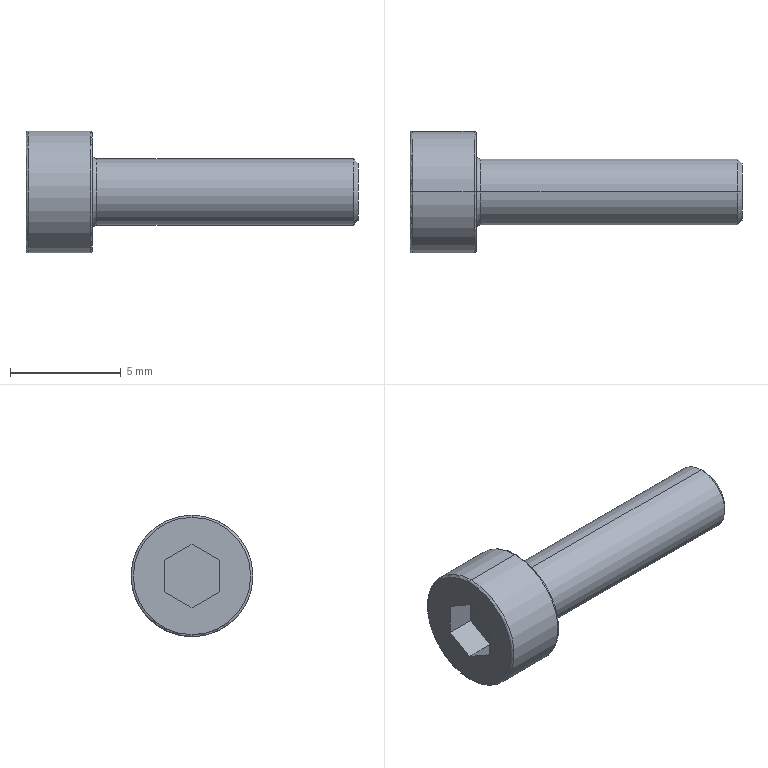Part | SolidWorks | features BlendCut 1, Chamfer 1, Cut 1, Fillet 1, Revolution 1 | 1 solid | 22 faces | box 15 x 5.5 x 5.5 mm | volume 148.972 mm3 | plane 10 | torus 6 | cylinder 4 | cone 2 | commonest cylinder face diameters 3 x2 5.5 x2
STEP:
#1=CARTESIAN_POINT('',(15.,0.,-1.3));
#2=VERTEX_POINT('',#1);
#3=CARTESIAN_POINT('',(15.,0.,1.3));
#4=VERTEX_POINT('',#3);
#5=CARTESIAN_POINT('',(15.,0.,0.));
#6=DIRECTION('',(1.,0.,0.));
#7=DIRECTION('',(0.,0.,1.));
#8=AXIS2_PLACEMENT_3D('',#5,#6,#7);
#9=CIRCLE('',#8,1.3);
#10=EDGE_CURVE('',#2,#4,#9,.T.);
#11=ORIENTED_EDGE('',*,*,#10,.F.);
#12=CARTESIAN_POINT('',(14.8,0.,-1.5));
#13=VERTEX_POINT('',#12);
#14=CARTESIAN_POINT('',(14.8,0.,-1.5));
#15=DIRECTION('',(-0.7071,0.,-0.7071));
#16=VECTOR('',#15,1000.);
#17=LINE('',#14,#16);
#18=EDGE_CURVE('',#2,#13,#17,.T.);
#19=ORIENTED_EDGE('',*,*,#18,.T.);
#20=CARTESIAN_POINT('',(14.8,0.,1.5));
#21=VERTEX_POINT('',#20);
#22=CARTESIAN_POINT('',(14.8,0.,0.));
#23=DIRECTION('',(-1.,0.,0.));
#24=DIRECTION('',(0.,0.,1.));
#25=AXIS2_PLACEMENT_3D('',#22,#23,#24);
#26=CIRCLE('',#25,1.5);
#27=EDGE_CURVE('',#21,#13,#26,.T.);
#28=ORIENTED_EDGE('',*,*,#27,.F.);
#29=CARTESIAN_POINT('',(14.8,0.,1.5));
#30=DIRECTION('',(-0.7071,0.,0.7071));
#31=VECTOR('',#30,1000.);
#32=LINE('',#29,#31);
#33=EDGE_CURVE('',#4,#21,#32,.T.);
#34=ORIENTED_EDGE('',*,*,#33,.F.);
#35=EDGE_LOOP('',(#11,#19,#28,#34));
#36=FACE_OUTER_BOUND('',#35,.T.);
#37=CARTESIAN_POINT('',(14.8,0.,0.));
#38=DIRECTION('',(-1.,0.,0.));
#39=DIRECTION('',(0.,0.,1.));
#40=AXIS2_PLACEMENT_3D('',#37,#38,#39);
#41=CONICAL_SURFACE('',#40,1.5,0.7854);
#42=ADVANCED_FACE('',(#36),#41,.T.);
#43=CARTESIAN_POINT('',(0.,0.,2.65));
#44=VERTEX_POINT('',#43);
#45=CARTESIAN_POINT('',(0.,0.,-2.65));
#46=VERTEX_POINT('',#45);
#47=CARTESIAN_POINT('',(0.,0.,0.));
#48=DIRECTION('',(-1.,0.,0.));
#49=DIRECTION('',(0.,0.,-1.));
#50=AXIS2_PLACEMENT_3D('',#47,#48,#49);
#51=CIRCLE('',#50,2.65);
#52=EDGE_CURVE('',#44,#46,#51,.T.);
#53=ORIENTED_EDGE('',*,*,#52,.F.);
#54=CARTESIAN_POINT('',(0.1,0.,2.75));
#55=VERTEX_POINT('',#54);
#56=CARTESIAN_POINT('',(0.1,0.,2.65));
#57=DIRECTION('',(0.,1.,0.));
#58=DIRECTION('',(0.,0.,1.));
#59=AXIS2_PLACEMENT_3D('',#56,#57,#58);
#60=CIRCLE('',#59,0.1);
#61=EDGE_CURVE('',#44,#55,#60,.T.);
#62=ORIENTED_EDGE('',*,*,#61,.T.);
#63=CARTESIAN_POINT('',(0.1,0.,-2.75));
#64=VERTEX_POINT('',#63);
#65=CARTESIAN_POINT('',(0.1,0.,0.));
#66=DIRECTION('',(1.,0.,0.));
#67=DIRECTION('',(0.,0.,-1.));
#68=AXIS2_PLACEMENT_3D('',#65,#66,#67);
#69=CIRCLE('',#68,2.75);
#70=EDGE_CURVE('',#64,#55,#69,.T.);
#71=ORIENTED_EDGE('',*,*,#70,.F.);
#72=CARTESIAN_POINT('',(0.1,0.,-2.65));
#73=DIRECTION('',(0.,-1.,0.));
#74=DIRECTION('',(0.,0.,-1.));
#75=AXIS2_PLACEMENT_3D('',#72,#73,#74);
#76=CIRCLE('',#75,0.1);
#77=EDGE_CURVE('',#46,#64,#76,.T.);
#78=ORIENTED_EDGE('',*,*,#77,.F.);
#79=EDGE_LOOP('',(#53,#62,#71,#78));
#80=FACE_OUTER_BOUND('',#79,.T.);
#81=CARTESIAN_POINT('',(0.1,0.,0.));
#82=DIRECTION('',(1.,0.,0.));
#83=DIRECTION('',(0.,0.,-1.));
#84=AXIS2_PLACEMENT_3D('',#81,#82,#83);
#85=TOROIDAL_SURFACE('',#84,2.65,0.1);
#86=ADVANCED_FACE('',(#80),#85,.T.);
#87=CARTESIAN_POINT('',(3.,0.,-2.65));
#88=VERTEX_POINT('',#87);
#89=CARTESIAN_POINT('',(3.,0.,2.65));
#90=VERTEX_POINT('',#89);
#91=CARTESIAN_POINT('',(3.,0.,0.));
#92=DIRECTION('',(1.,0.,0.));
#93=DIRECTION('',(0.,0.,1.));
#94=AXIS2_PLACEMENT_3D('',#91,#92,#93);
#95=CIRCLE('',#94,2.65);
#96=EDGE_CURVE('',#88,#90,#95,.T.);
#97=ORIENTED_EDGE('',*,*,#96,.F.);
#98=CARTESIAN_POINT('',(2.9,0.,-2.75));
#99=VERTEX_POINT('',#98);
#100=CARTESIAN_POINT('',(2.9,0.,-2.65));
#101=DIRECTION('',(0.,1.,0.));
#102=DIRECTION('',(0.,0.,1.));
#103=AXIS2_PLACEMENT_3D('',#100,#101,#102);
#104=CIRCLE('',#103,0.1);
#105=EDGE_CURVE('',#88,#99,#104,.T.);
#106=ORIENTED_EDGE('',*,*,#105,.T.);
#107=CARTESIAN_POINT('',(2.9,0.,2.75));
#108=VERTEX_POINT('',#107);
#109=CARTESIAN_POINT('',(2.9,0.,0.));
#110=DIRECTION('',(-1.,0.,0.));
#111=DIRECTION('',(0.,0.,1.));
#112=AXIS2_PLACEMENT_3D('',#109,#110,#111);
#113=CIRCLE('',#112,2.75);
#114=EDGE_CURVE('',#108,#99,#113,.T.);
#115=ORIENTED_EDGE('',*,*,#114,.F.);
#116=CARTESIAN_POINT('',(2.9,0.,2.65));
#117=DIRECTION('',(0.,-1.,0.));
#118=DIRECTION('',(0.,0.,-1.));
#119=AXIS2_PLACEMENT_3D('',#116,#117,#118);
#120=CIRCLE('',#119,0.1);
#121=EDGE_CURVE('',#90,#108,#120,.T.);
#122=ORIENTED_EDGE('',*,*,#121,.F.);
#123=EDGE_LOOP('',(#97,#106,#115,#122));
#124=FACE_OUTER_BOUND('',#123,.T.);
#125=CARTESIAN_POINT('',(2.9,0.,0.));
#126=DIRECTION('',(-1.,0.,0.));
#127=DIRECTION('',(0.,0.,1.));
#128=AXIS2_PLACEMENT_3D('',#125,#126,#127);
#129=TOROIDAL_SURFACE('',#128,2.65,0.1);
#130=ADVANCED_FACE('',(#124),#129,.T.);
#131=ORIENTED_EDGE('',*,*,#27,.T.);
#132=CARTESIAN_POINT('',(3.2,0.,-1.5));
#133=VERTEX_POINT('',#132);
#134=CARTESIAN_POINT('',(0.,0.,-1.5));
#135=DIRECTION('',(-1.,0.,0.));
#136=VECTOR('',#135,1000.);
#137=LINE('',#134,#136);
#138=EDGE_CURVE('',#13,#133,#137,.T.);
#139=ORIENTED_EDGE('',*,*,#138,.T.);
#140=CARTESIAN_POINT('',(3.2,0.,1.5));
#141=VERTEX_POINT('',#140);
#142=CARTESIAN_POINT('',(3.2,0.,0.));
#143=DIRECTION('',(-1.,0.,0.));
#144=DIRECTION('',(0.,0.,1.));
#145=AXIS2_PLACEMENT_3D('',#142,#143,#144);
#146=CIRCLE('',#145,1.5);
#147=EDGE_CURVE('',#141,#133,#146,.T.);
#148=ORIENTED_EDGE('',*,*,#147,.F.);
#149=CARTESIAN_POINT('',(0.,0.,1.5));
#150=DIRECTION('',(-1.,0.,0.));
#151=VECTOR('',#150,1000.);
#152=LINE('',#149,#151);
#153=EDGE_CURVE('',#21,#141,#152,.T.);
#154=ORIENTED_EDGE('',*,*,#153,.F.);
#155=EDGE_LOOP('',(#131,#139,#148,#154));
#156=FACE_OUTER_BOUND('',#155,.T.);
#157=CARTESIAN_POINT('',(0.,0.,0.));
#158=DIRECTION('',(-1.,0.,0.));
#159=DIRECTION('',(0.,0.,1.));
#160=AXIS2_PLACEMENT_3D('',#157,#158,#159);
#161=CYLINDRICAL_SURFACE('',#160,1.5);
#162=ADVANCED_FACE('',(#156),#161,.T.);
#163=CARTESIAN_POINT('',(3.,0.,-1.7));
#164=VERTEX_POINT('',#163);
#165=CARTESIAN_POINT('',(3.,0.,1.7));
#166=VERTEX_POINT('',#165);
#167=CARTESIAN_POINT('',(3.,0.,0.));
#168=DIRECTION('',(-1.,0.,0.));
#169=DIRECTION('',(0.,0.,1.));
#170=AXIS2_PLACEMENT_3D('',#167,#168,#169);
#171=CIRCLE('',#170,1.7);
#172=EDGE_CURVE('',#164,#166,#171,.T.);
#173=ORIENTED_EDGE('',*,*,#172,.F.);
#174=CARTESIAN_POINT('',(3.2,0.,-1.7));
#175=DIRECTION('',(0.,1.,0.));
#176=DIRECTION('',(0.,0.,1.));
#177=AXIS2_PLACEMENT_3D('',#174,#175,#176);
#178=CIRCLE('',#177,0.2);
#179=EDGE_CURVE('',#164,#133,#178,.T.);
#180=ORIENTED_EDGE('',*,*,#179,.T.);
#181=CARTESIAN_POINT('',(3.2,0.,0.));
#182=DIRECTION('',(-1.,0.,0.));
#183=DIRECTION('',(0.,0.,1.));
#184=AXIS2_PLACEMENT_3D('',#181,#182,#183);
#185=CIRCLE('',#184,1.5);
#186=EDGE_CURVE('',#133,#141,#185,.T.);
#187=ORIENTED_EDGE('',*,*,#186,.T.);
#188=CARTESIAN_POINT('',(3.2,0.,1.7));
#189=DIRECTION('',(0.,-1.,0.));
#190=DIRECTION('',(0.,0.,-1.));
#191=AXIS2_PLACEMENT_3D('',#188,#189,#190);
#192=CIRCLE('',#191,0.2);
#193=EDGE_CURVE('',#166,#141,#192,.T.);
#194=ORIENTED_EDGE('',*,*,#193,.F.);
#195=EDGE_LOOP('',(#173,#180,#187,#194));
#196=FACE_OUTER_BOUND('',#195,.T.);
#197=CARTESIAN_POINT('',(3.2,0.,0.));
#198=DIRECTION('',(-1.,0.,0.));
#199=DIRECTION('',(0.,0.,1.));
#200=AXIS2_PLACEMENT_3D('',#197,#198,#199);
#201=TOROIDAL_SURFACE('',#200,1.7,0.2);
#202=ADVANCED_FACE('',(#196),#201,.F.);
#203=ORIENTED_EDGE('',*,*,#114,.T.);
#204=CARTESIAN_POINT('',(0.,0.,-2.75));
#205=DIRECTION('',(-1.,0.,0.));
#206=VECTOR('',#205,1000.);
#207=LINE('',#204,#206);
#208=EDGE_CURVE('',#99,#64,#207,.T.);
#209=ORIENTED_EDGE('',*,*,#208,.T.);
#210=ORIENTED_EDGE('',*,*,#70,.T.);
#211=CARTESIAN_POINT('',(0.,0.,2.75));
#212=DIRECTION('',(-1.,0.,0.));
#213=VECTOR('',#212,1000.);
#214=LINE('',#211,#213);
#215=EDGE_CURVE('',#108,#55,#214,.T.);
#216=ORIENTED_EDGE('',*,*,#215,.F.);
#217=EDGE_LOOP('',(#203,#209,#210,#216));
#218=FACE_OUTER_BOUND('',#217,.T.);
#219=CARTESIAN_POINT('',(0.,0.,0.));
#220=DIRECTION('',(-1.,0.,0.));
#221=DIRECTION('',(0.,0.,1.));
#222=AXIS2_PLACEMENT_3D('',#219,#220,#221);
#223=CYLINDRICAL_SURFACE('',#222,2.75);
#224=ADVANCED_FACE('',(#218),#223,.T.);
#225=CARTESIAN_POINT('',(0.,0.,0.));
#226=DIRECTION('',(-1.,0.,0.));
#227=DIRECTION('',(0.,0.,-1.));
#228=AXIS2_PLACEMENT_3D('',#225,#226,#227);
#229=CIRCLE('',#228,2.65);
#230=EDGE_CURVE('',#46,#44,#229,.T.);
#231=ORIENTED_EDGE('',*,*,#230,.T.);
#232=ORIENTED_EDGE('',*,*,#52,.T.);
#233=EDGE_LOOP('',(#231,#232));
#234=FACE_OUTER_BOUND('',#233,.T.);
#235=CARTESIAN_POINT('',(0.,0.,1.435));
#236=VERTEX_POINT('',#235);
#237=CARTESIAN_POINT('',(0.,1.243,0.7175));
#238=VERTEX_POINT('',#237);
#239=CARTESIAN_POINT('',(0.,0.,1.435));
#240=DIRECTION('',(0.,0.866,-0.5));
#241=VECTOR('',#240,1000.);
#242=LINE('',#239,#241);
#243=EDGE_CURVE('',#236,#238,#242,.T.);
#244=ORIENTED_EDGE('',*,*,#243,.F.);
#245=CARTESIAN_POINT('',(0.,-1.243,0.7175));
#246=VERTEX_POINT('',#245);
#247=CARTESIAN_POINT('',(0.,-1.243,0.7175));
#248=DIRECTION('',(0.,0.866,0.5));
#249=VECTOR('',#248,1000.);
#250=LINE('',#247,#249);
#251=EDGE_CURVE('',#246,#236,#250,.T.);
#252=ORIENTED_EDGE('',*,*,#251,.F.);
#253=CARTESIAN_POINT('',(0.,-1.243,-0.7175));
#254=VERTEX_POINT('',#253);
#255=CARTESIAN_POINT('',(0.,-1.243,-0.7175));
#256=DIRECTION('',(0.,0.,1.));
#257=VECTOR('',#256,1000.);
#258=LINE('',#255,#257);
#259=EDGE_CURVE('',#254,#246,#258,.T.);
#260=ORIENTED_EDGE('',*,*,#259,.F.);
#261=CARTESIAN_POINT('',(0.,0.,-1.435));
#262=VERTEX_POINT('',#261);
#263=CARTESIAN_POINT('',(0.,0.,-1.435));
#264=DIRECTION('',(0.,-0.866,0.5));
#265=VECTOR('',#264,1000.);
#266=LINE('',#263,#265);
#267=EDGE_CURVE('',#262,#254,#266,.T.);
#268=ORIENTED_EDGE('',*,*,#267,.F.);
#269=CARTESIAN_POINT('',(0.,1.243,-0.7175));
#270=VERTEX_POINT('',#269);
#271=CARTESIAN_POINT('',(0.,1.243,-0.7175));
#272=DIRECTION('',(0.,-0.866,-0.5));
#273=VECTOR('',#272,1000.);
#274=LINE('',#271,#273);
#275=EDGE_CURVE('',#270,#262,#274,.T.);
#276=ORIENTED_EDGE('',*,*,#275,.F.);
#277=CARTESIAN_POINT('',(0.,1.243,0.7175));
#278=DIRECTION('',(0.,0.,-1.));
#279=VECTOR('',#278,1000.);
#280=LINE('',#277,#279);
#281=EDGE_CURVE('',#238,#270,#280,.T.);
#282=ORIENTED_EDGE('',*,*,#281,.F.);
#283=EDGE_LOOP('',(#244,#252,#260,#268,#276,#282));
#284=FACE_BOUND('',#283,.T.);
#285=CARTESIAN_POINT('',(0.,0.,0.));
#286=DIRECTION('',(1.,0.,0.));
#287=DIRECTION('',(0.,0.,-1.));
#288=AXIS2_PLACEMENT_3D('',#285,#286,#287);
#289=PLANE('',#288);
#290=ADVANCED_FACE('',(#234,#284),#289,.F.);
#291=ORIENTED_EDGE('',*,*,#208,.F.);
#292=CARTESIAN_POINT('',(2.9,0.,0.));
#293=DIRECTION('',(-1.,0.,0.));
#294=DIRECTION('',(0.,0.,1.));
#295=AXIS2_PLACEMENT_3D('',#292,#293,#294);
#296=CIRCLE('',#295,2.75);
#297=EDGE_CURVE('',#99,#108,#296,.T.);
#298=ORIENTED_EDGE('',*,*,#297,.T.);
#299=ORIENTED_EDGE('',*,*,#215,.T.);
#300=CARTESIAN_POINT('',(0.1,0.,0.));
#301=DIRECTION('',(1.,0.,0.));
#302=DIRECTION('',(0.,0.,-1.));
#303=AXIS2_PLACEMENT_3D('',#300,#301,#302);
#304=CIRCLE('',#303,2.75);
#305=EDGE_CURVE('',#55,#64,#304,.T.);
#306=ORIENTED_EDGE('',*,*,#305,.T.);
#307=EDGE_LOOP('',(#291,#298,#299,#306));
#308=FACE_OUTER_BOUND('',#307,.T.);
#309=CARTESIAN_POINT('',(0.,0.,0.));
#310=DIRECTION('',(-1.,0.,0.));
#311=DIRECTION('',(0.,0.,1.));
#312=AXIS2_PLACEMENT_3D('',#309,#310,#311);
#313=CYLINDRICAL_SURFACE('',#312,2.75);
#314=ADVANCED_FACE('',(#308),#313,.T.);
#315=CARTESIAN_POINT('',(3.,0.,0.));
#316=DIRECTION('',(1.,0.,0.));
#317=DIRECTION('',(0.,0.,1.));
#318=AXIS2_PLACEMENT_3D('',#315,#316,#317);
#319=CIRCLE('',#318,2.65);
#320=EDGE_CURVE('',#90,#88,#319,.T.);
#321=ORIENTED_EDGE('',*,*,#320,.T.);
#322=ORIENTED_EDGE('',*,*,#96,.T.);
#323=EDGE_LOOP('',(#321,#322));
#324=FACE_OUTER_BOUND('',#323,.T.);
#325=CARTESIAN_POINT('',(3.,0.,0.));
#326=DIRECTION('',(-1.,0.,0.));
#327=DIRECTION('',(0.,0.,1.));
#328=AXIS2_PLACEMENT_3D('',#325,#326,#327);
#329=CIRCLE('',#328,1.7);
#330=EDGE_CURVE('',#166,#164,#329,.T.);
#331=ORIENTED_EDGE('',*,*,#330,.T.);
#332=ORIENTED_EDGE('',*,*,#172,.T.);
#333=EDGE_LOOP('',(#331,#332));
#334=FACE_BOUND('',#333,.T.);
#335=CARTESIAN_POINT('',(3.,2.75,0.));
#336=DIRECTION('',(-1.,0.,0.));
#337=DIRECTION('',(0.,0.,1.));
#338=AXIS2_PLACEMENT_3D('',#335,#336,#337);
#339=PLANE('',#338);
#340=ADVANCED_FACE('',(#324,#334),#339,.F.);
#341=ORIENTED_EDGE('',*,*,#179,.F.);
#342=ORIENTED_EDGE('',*,*,#330,.F.);
#343=ORIENTED_EDGE('',*,*,#193,.T.);
#344=ORIENTED_EDGE('',*,*,#147,.T.);
#345=EDGE_LOOP('',(#341,#342,#343,#344));
#346=FACE_OUTER_BOUND('',#345,.T.);
#347=CARTESIAN_POINT('',(3.2,0.,0.));
#348=DIRECTION('',(-1.,0.,0.));
#349=DIRECTION('',(0.,0.,1.));
#350=AXIS2_PLACEMENT_3D('',#347,#348,#349);
#351=TOROIDAL_SURFACE('',#350,1.7,0.2);
#352=ADVANCED_FACE('',(#346),#351,.F.);
#353=ORIENTED_EDGE('',*,*,#138,.F.);
#354=CARTESIAN_POINT('',(14.8,0.,0.));
#355=DIRECTION('',(-1.,0.,0.));
#356=DIRECTION('',(0.,0.,1.));
#357=AXIS2_PLACEMENT_3D('',#354,#355,#356);
#358=CIRCLE('',#357,1.5);
#359=EDGE_CURVE('',#13,#21,#358,.T.);
#360=ORIENTED_EDGE('',*,*,#359,.T.);
#361=ORIENTED_EDGE('',*,*,#153,.T.);
#362=ORIENTED_EDGE('',*,*,#186,.F.);
#363=EDGE_LOOP('',(#353,#360,#361,#362));
#364=FACE_OUTER_BOUND('',#363,.T.);
#365=CARTESIAN_POINT('',(0.,0.,0.));
#366=DIRECTION('',(-1.,0.,0.));
#367=DIRECTION('',(0.,0.,1.));
#368=AXIS2_PLACEMENT_3D('',#365,#366,#367);
#369=CYLINDRICAL_SURFACE('',#368,1.5);
#370=ADVANCED_FACE('',(#364),#369,.T.);
#371=CARTESIAN_POINT('',(15.,0.,0.));
#372=DIRECTION('',(1.,0.,0.));
#373=DIRECTION('',(0.,0.,1.));
#374=AXIS2_PLACEMENT_3D('',#371,#372,#373);
#375=CIRCLE('',#374,1.3);
#376=EDGE_CURVE('',#4,#2,#375,.T.);
#377=ORIENTED_EDGE('',*,*,#376,.T.);
#378=ORIENTED_EDGE('',*,*,#10,.T.);
#379=EDGE_LOOP('',(#377,#378));
#380=FACE_OUTER_BOUND('',#379,.T.);
#381=CARTESIAN_POINT('',(15.,1.5,0.));
#382=DIRECTION('',(-1.,0.,0.));
#383=DIRECTION('',(0.,0.,1.));
#384=AXIS2_PLACEMENT_3D('',#381,#382,#383);
#385=PLANE('',#384);
#386=ADVANCED_FACE('',(#380),#385,.F.);
#387=ORIENTED_EDGE('',*,*,#251,.T.);
#388=CARTESIAN_POINT('',(1.3,0.,1.435));
#389=VERTEX_POINT('',#388);
#390=CARTESIAN_POINT('',(1.3,0.,1.435));
#391=DIRECTION('',(-1.,0.,0.));
#392=VECTOR('',#391,1000.);
#393=LINE('',#390,#392);
#394=EDGE_CURVE('',#389,#236,#393,.T.);
#395=ORIENTED_EDGE('',*,*,#394,.F.);
#396=CARTESIAN_POINT('',(1.3,-1.243,0.7175));
#397=VERTEX_POINT('',#396);
#398=CARTESIAN_POINT('',(1.3,-1.243,0.7175));
#399=DIRECTION('',(0.,0.866,0.5));
#400=VECTOR('',#399,1000.);
#401=LINE('',#398,#400);
#402=EDGE_CURVE('',#397,#389,#401,.T.);
#403=ORIENTED_EDGE('',*,*,#402,.F.);
#404=CARTESIAN_POINT('',(1.3,-1.243,0.7175));
#405=DIRECTION('',(-1.,0.,0.));
#406=VECTOR('',#405,1000.);
#407=LINE('',#404,#406);
#408=EDGE_CURVE('',#397,#246,#407,.T.);
#409=ORIENTED_EDGE('',*,*,#408,.T.);
#410=EDGE_LOOP('',(#387,#395,#403,#409));
#411=FACE_OUTER_BOUND('',#410,.T.);
#412=CARTESIAN_POINT('',(1.3,-1.243,0.7175));
#413=DIRECTION('',(0.,-0.5,0.866));
#414=DIRECTION('',(0.,-0.866,-0.5));
#415=AXIS2_PLACEMENT_3D('',#412,#413,#414);
#416=PLANE('',#415);
#417=ADVANCED_FACE('',(#411),#416,.F.);
#418=ORIENTED_EDGE('',*,*,#259,.T.);
#419=ORIENTED_EDGE('',*,*,#408,.F.);
#420=CARTESIAN_POINT('',(1.3,-1.243,-0.7175));
#421=VERTEX_POINT('',#420);
#422=CARTESIAN_POINT('',(1.3,-1.243,-0.7175));
#423=DIRECTION('',(0.,0.,1.));
#424=VECTOR('',#423,1000.);
#425=LINE('',#422,#424);
#426=EDGE_CURVE('',#421,#397,#425,.T.);
#427=ORIENTED_EDGE('',*,*,#426,.F.);
#428=CARTESIAN_POINT('',(1.3,-1.243,-0.7175));
#429=DIRECTION('',(-1.,0.,0.));
#430=VECTOR('',#429,1000.);
#431=LINE('',#428,#430);
#432=EDGE_CURVE('',#421,#254,#431,.T.);
#433=ORIENTED_EDGE('',*,*,#432,.T.);
#434=EDGE_LOOP('',(#418,#419,#427,#433));
#435=FACE_OUTER_BOUND('',#434,.T.);
#436=CARTESIAN_POINT('',(1.3,-1.243,-0.7175));
#437=DIRECTION('',(0.,-1.,0.));
#438=DIRECTION('',(0.,0.,-1.));
#439=AXIS2_PLACEMENT_3D('',#436,#437,#438);
#440=PLANE('',#439);
#441=ADVANCED_FACE('',(#435),#440,.F.);
#442=ORIENTED_EDGE('',*,*,#267,.T.);
#443=ORIENTED_EDGE('',*,*,#432,.F.);
#444=CARTESIAN_POINT('',(1.3,0.,-1.435));
#445=VERTEX_POINT('',#444);
#446=CARTESIAN_POINT('',(1.3,0.,-1.435));
#447=DIRECTION('',(0.,-0.866,0.5));
#448=VECTOR('',#447,1000.);
#449=LINE('',#446,#448);
#450=EDGE_CURVE('',#445,#421,#449,.T.);
#451=ORIENTED_EDGE('',*,*,#450,.F.);
#452=CARTESIAN_POINT('',(1.3,0.,-1.435));
#453=DIRECTION('',(-1.,0.,0.));
#454=VECTOR('',#453,1000.);
#455=LINE('',#452,#454);
#456=EDGE_CURVE('',#445,#262,#455,.T.);
#457=ORIENTED_EDGE('',*,*,#456,.T.);
#458=EDGE_LOOP('',(#442,#443,#451,#457));
#459=FACE_OUTER_BOUND('',#458,.T.);
#460=CARTESIAN_POINT('',(1.3,0.,-1.435));
#461=DIRECTION('',(0.,-0.5,-0.866));
#462=DIRECTION('',(0.,0.866,-0.5));
#463=AXIS2_PLACEMENT_3D('',#460,#461,#462);
#464=PLANE('',#463);
#465=ADVANCED_FACE('',(#459),#464,.F.);
#466=ORIENTED_EDGE('',*,*,#275,.T.);
#467=ORIENTED_EDGE('',*,*,#456,.F.);
#468=CARTESIAN_POINT('',(1.3,1.243,-0.7175));
#469=VERTEX_POINT('',#468);
#470=CARTESIAN_POINT('',(1.3,1.243,-0.7175));
#471=DIRECTION('',(0.,-0.866,-0.5));
#472=VECTOR('',#471,1000.);
#473=LINE('',#470,#472);
#474=EDGE_CURVE('',#469,#445,#473,.T.);
#475=ORIENTED_EDGE('',*,*,#474,.F.);
#476=CARTESIAN_POINT('',(1.3,1.243,-0.7175));
#477=DIRECTION('',(-1.,0.,0.));
#478=VECTOR('',#477,1000.);
#479=LINE('',#476,#478);
#480=EDGE_CURVE('',#469,#270,#479,.T.);
#481=ORIENTED_EDGE('',*,*,#480,.T.);
#482=EDGE_LOOP('',(#466,#467,#475,#481));
#483=FACE_OUTER_BOUND('',#482,.T.);
#484=CARTESIAN_POINT('',(1.3,1.243,-0.7175));
#485=DIRECTION('',(0.,0.5,-0.866));
#486=DIRECTION('',(0.,0.866,0.5));
#487=AXIS2_PLACEMENT_3D('',#484,#485,#486);
#488=PLANE('',#487);
#489=ADVANCED_FACE('',(#483),#488,.F.);
#490=ORIENTED_EDGE('',*,*,#281,.T.);
#491=ORIENTED_EDGE('',*,*,#480,.F.);
#492=CARTESIAN_POINT('',(1.3,1.243,0.7175));
#493=VERTEX_POINT('',#492);
#494=CARTESIAN_POINT('',(1.3,1.243,0.7175));
#495=DIRECTION('',(0.,0.,-1.));
#496=VECTOR('',#495,1000.);
#497=LINE('',#494,#496);
#498=EDGE_CURVE('',#493,#469,#497,.T.);
#499=ORIENTED_EDGE('',*,*,#498,.F.);
#500=CARTESIAN_POINT('',(1.3,1.243,0.7175));
#501=DIRECTION('',(-1.,0.,0.));
#502=VECTOR('',#501,1000.);
#503=LINE('',#500,#502);
#504=EDGE_CURVE('',#493,#238,#503,.T.);
#505=ORIENTED_EDGE('',*,*,#504,.T.);
#506=EDGE_LOOP('',(#490,#491,#499,#505));
#507=FACE_OUTER_BOUND('',#506,.T.);
#508=CARTESIAN_POINT('',(1.3,1.243,0.7175));
#509=DIRECTION('',(0.,1.,0.));
#510=DIRECTION('',(0.,0.,1.));
#511=AXIS2_PLACEMENT_3D('',#508,#509,#510);
#512=PLANE('',#511);
#513=ADVANCED_FACE('',(#507),#512,.F.);
#514=ORIENTED_EDGE('',*,*,#243,.T.);
#515=ORIENTED_EDGE('',*,*,#504,.F.);
#516=CARTESIAN_POINT('',(1.3,0.,1.435));
#517=DIRECTION('',(0.,0.866,-0.5));
#518=VECTOR('',#517,1000.);
#519=LINE('',#516,#518);
#520=EDGE_CURVE('',#389,#493,#519,.T.);
#521=ORIENTED_EDGE('',*,*,#520,.F.);
#522=ORIENTED_EDGE('',*,*,#394,.T.);
#523=EDGE_LOOP('',(#514,#515,#521,#522));
#524=FACE_OUTER_BOUND('',#523,.T.);
#525=CARTESIAN_POINT('',(1.3,0.,1.435));
#526=DIRECTION('',(0.,0.5,0.866));
#527=DIRECTION('',(0.,-0.866,0.5));
#528=AXIS2_PLACEMENT_3D('',#525,#526,#527);
#529=PLANE('',#528);
#530=ADVANCED_FACE('',(#524),#529,.F.);
#531=ORIENTED_EDGE('',*,*,#402,.T.);
#532=ORIENTED_EDGE('',*,*,#520,.T.);
#533=ORIENTED_EDGE('',*,*,#498,.T.);
#534=ORIENTED_EDGE('',*,*,#474,.T.);
#535=ORIENTED_EDGE('',*,*,#450,.T.);
#536=ORIENTED_EDGE('',*,*,#426,.T.);
#537=EDGE_LOOP('',(#531,#532,#533,#534,#535,#536));
#538=FACE_OUTER_BOUND('',#537,.T.);
#539=CARTESIAN_POINT('',(1.3,-1.243,0.7175));
#540=DIRECTION('',(1.,0.,0.));
#541=DIRECTION('',(0.,0.,-1.));
#542=AXIS2_PLACEMENT_3D('',#539,#540,#541);
#543=PLANE('',#542);
#544=ADVANCED_FACE('',(#538),#543,.F.);
#545=ORIENTED_EDGE('',*,*,#105,.F.);
#546=ORIENTED_EDGE('',*,*,#320,.F.);
#547=ORIENTED_EDGE('',*,*,#121,.T.);
#548=ORIENTED_EDGE('',*,*,#297,.F.);
#549=EDGE_LOOP('',(#545,#546,#547,#548));
#550=FACE_OUTER_BOUND('',#549,.T.);
#551=CARTESIAN_POINT('',(2.9,0.,0.));
#552=DIRECTION('',(-1.,0.,0.));
#553=DIRECTION('',(0.,0.,1.));
#554=AXIS2_PLACEMENT_3D('',#551,#552,#553);
#555=TOROIDAL_SURFACE('',#554,2.65,0.1);
#556=ADVANCED_FACE('',(#550),#555,.T.);
#557=ORIENTED_EDGE('',*,*,#61,.F.);
#558=ORIENTED_EDGE('',*,*,#230,.F.);
#559=ORIENTED_EDGE('',*,*,#77,.T.);
#560=ORIENTED_EDGE('',*,*,#305,.F.);
#561=EDGE_LOOP('',(#557,#558,#559,#560));
#562=FACE_OUTER_BOUND('',#561,.T.);
#563=CARTESIAN_POINT('',(0.1,0.,0.));
#564=DIRECTION('',(1.,0.,0.));
#565=DIRECTION('',(0.,0.,-1.));
#566=AXIS2_PLACEMENT_3D('',#563,#564,#565);
#567=TOROIDAL_SURFACE('',#566,2.65,0.1);
#568=ADVANCED_FACE('',(#562),#567,.T.);
#569=ORIENTED_EDGE('',*,*,#18,.F.);
#570=ORIENTED_EDGE('',*,*,#376,.F.);
#571=ORIENTED_EDGE('',*,*,#33,.T.);
#572=ORIENTED_EDGE('',*,*,#359,.F.);
#573=EDGE_LOOP('',(#569,#570,#571,#572));
#574=FACE_OUTER_BOUND('',#573,.T.);
#575=CARTESIAN_POINT('',(14.8,0.,0.));
#576=DIRECTION('',(-1.,0.,0.));
#577=DIRECTION('',(0.,0.,1.));
#578=AXIS2_PLACEMENT_3D('',#575,#576,#577);
#579=CONICAL_SURFACE('',#578,1.5,0.7854);
#580=ADVANCED_FACE('',(#574),#579,.T.);
#581=CLOSED_SHELL('',(#42,#86,#130,#162,#202,#224,#290,#314,#340,#352,#370,#386,#417,#441,#465,#489,#513,#530,#544,#556,#568,#580));
#582=MANIFOLD_SOLID_BREP('',#581);
#583=CARTESIAN_POINT('',(0.,0.,0.));
#584=DIRECTION('',(0.,0.,1.));
#585=DIRECTION('',(1.,0.,0.));
#586=AXIS2_PLACEMENT_3D('',#583,#584,#585);
#587=(LENGTH_UNIT()NAMED_UNIT(*)SI_UNIT(.MILLI.,.METRE.));
#588=UNCERTAINTY_MEASURE_WITH_UNIT(LENGTH_MEASURE(0.00001),#587,'','');
#589=(NAMED_UNIT(*)PLANE_ANGLE_UNIT()SI_UNIT($,.RADIAN.));
#590=(NAMED_UNIT(*)SI_UNIT($,.STERADIAN.)SOLID_ANGLE_UNIT());
#591=(GEOMETRIC_REPRESENTATION_CONTEXT(3)GLOBAL_UNCERTAINTY_ASSIGNED_CONTEXT((#588))GLOBAL_UNIT_ASSIGNED_CONTEXT((#587,#589,#590))REPRESENTATION_CONTEXT('',''));
#592=ADVANCED_BREP_SHAPE_REPRESENTATION('',(#582,#586),#591);